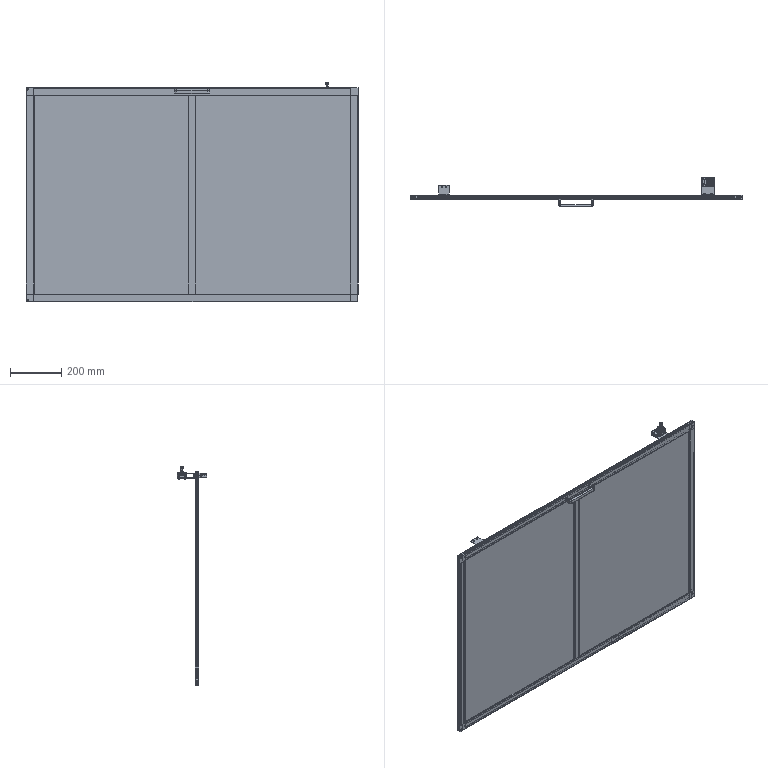Part | SolidWorks | features LocalLPattern 3, ReferencePattern 3, CompositeCurve 2 | 43 solids | 2288 faces | box 1296 x 114.543 x 856.55 mm | volume 6140748 mm3 | plane 1109 | cylinder 586 | cone 366 | spline 128 | torus 87 | sphere 12 | commonest cylinder face diameters 1 x83 5 x73 11 x52 4.5 x40 6.5 x28 2 x26